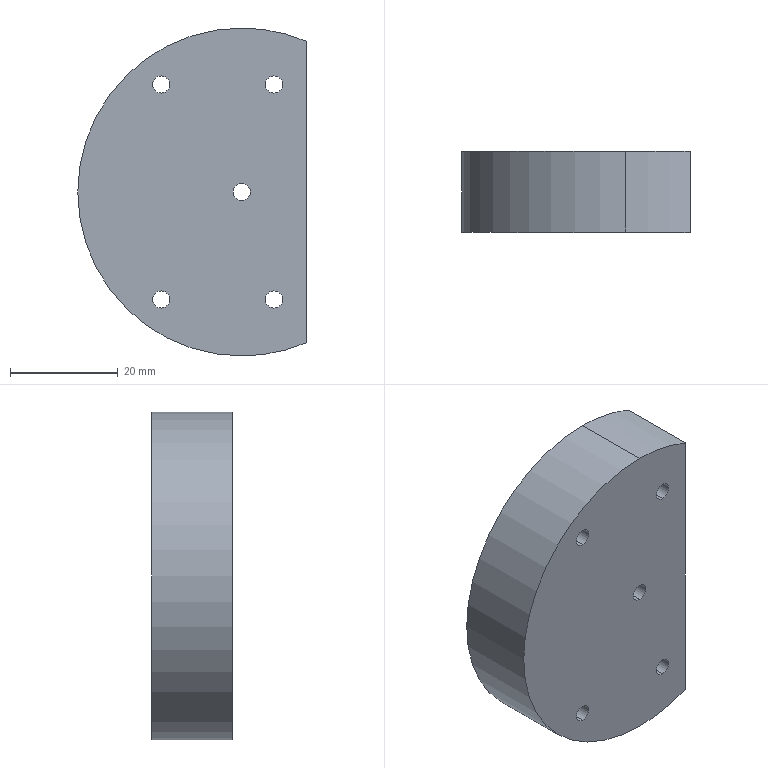Part | SolidWorks | features BaseBody 1 | 1 solid | 23 faces | box 42.5 x 15 x 61 mm | volume 7856 mm3 | cylinder 16 | plane 4 | spline 3 | commonest cylinder face diameters 3.2 x10 59 x3 61 x3
STEP:
#1=CARTESIAN_POINT('',(-15.,0.,21.6));
#2=VERTEX_POINT('',#1);
#3=CARTESIAN_POINT('',(-15.,0.,18.4));
#4=VERTEX_POINT('',#3);
#5=CARTESIAN_POINT('',(-15.,0.,20.));
#6=DIRECTION('',(0.,-1.,0.));
#7=DIRECTION('',(0.,0.,1.));
#8=AXIS2_PLACEMENT_3D('',#5,#6,#7);
#9=CIRCLE('',#8,1.6);
#10=EDGE_CURVE('',#2,#4,#9,.T.);
#11=ORIENTED_EDGE('',*,*,#10,.T.);
#12=CARTESIAN_POINT('',(-15.,3.,18.4));
#13=VERTEX_POINT('',#12);
#14=CARTESIAN_POINT('',(-15.,0.,18.4));
#15=DIRECTION('',(0.,1.,0.));
#16=VECTOR('',#15,1000.);
#17=LINE('',#14,#16);
#18=EDGE_CURVE('',#4,#13,#17,.T.);
#19=ORIENTED_EDGE('',*,*,#18,.T.);
#20=CARTESIAN_POINT('',(-15.,3.,21.6));
#21=VERTEX_POINT('',#20);
#22=CARTESIAN_POINT('',(-15.,3.,20.));
#23=DIRECTION('',(0.,1.,0.));
#24=DIRECTION('',(0.,0.,1.));
#25=AXIS2_PLACEMENT_3D('',#22,#23,#24);
#26=CIRCLE('',#25,1.6);
#27=EDGE_CURVE('',#13,#21,#26,.T.);
#28=ORIENTED_EDGE('',*,*,#27,.T.);
#29=CARTESIAN_POINT('',(-15.,0.,21.6));
#30=DIRECTION('',(0.,1.,0.));
#31=VECTOR('',#30,1000.);
#32=LINE('',#29,#31);
#33=EDGE_CURVE('',#2,#21,#32,.T.);
#34=ORIENTED_EDGE('',*,*,#33,.F.);
#35=EDGE_LOOP('',(#11,#19,#28,#34));
#36=FACE_OUTER_BOUND('',#35,.T.);
#37=CARTESIAN_POINT('',(-15.,0.,20.));
#38=DIRECTION('',(0.,1.,0.));
#39=DIRECTION('',(0.,0.,1.));
#40=AXIS2_PLACEMENT_3D('',#37,#38,#39);
#41=CYLINDRICAL_SURFACE('',#40,1.6);
#42=ADVANCED_FACE('',(#36),#41,.F.);
#43=CARTESIAN_POINT('',(6.,0.,18.4));
#44=VERTEX_POINT('',#43);
#45=CARTESIAN_POINT('',(6.,0.,21.6));
#46=VERTEX_POINT('',#45);
#47=CARTESIAN_POINT('',(6.,0.,20.));
#48=DIRECTION('',(0.,1.,0.));
#49=DIRECTION('',(0.,0.,1.));
#50=AXIS2_PLACEMENT_3D('',#47,#48,#49);
#51=CIRCLE('',#50,1.6);
#52=EDGE_CURVE('',#44,#46,#51,.T.);
#53=ORIENTED_EDGE('',*,*,#52,.F.);
#54=CARTESIAN_POINT('',(6.,3.,18.4));
#55=VERTEX_POINT('',#54);
#56=CARTESIAN_POINT('',(6.,0.,18.4));
#57=DIRECTION('',(0.,1.,0.));
#58=VECTOR('',#57,1000.);
#59=LINE('',#56,#58);
#60=EDGE_CURVE('',#44,#55,#59,.T.);
#61=ORIENTED_EDGE('',*,*,#60,.T.);
#62=CARTESIAN_POINT('',(6.,3.,21.6));
#63=VERTEX_POINT('',#62);
#64=CARTESIAN_POINT('',(6.,3.,20.));
#65=DIRECTION('',(0.,-1.,0.));
#66=DIRECTION('',(0.,0.,1.));
#67=AXIS2_PLACEMENT_3D('',#64,#65,#66);
#68=CIRCLE('',#67,1.6);
#69=EDGE_CURVE('',#63,#55,#68,.T.);
#70=ORIENTED_EDGE('',*,*,#69,.F.);
#71=CARTESIAN_POINT('',(6.,0.,21.6));
#72=DIRECTION('',(0.,1.,0.));
#73=VECTOR('',#72,1000.);
#74=LINE('',#71,#73);
#75=EDGE_CURVE('',#46,#63,#74,.T.);
#76=ORIENTED_EDGE('',*,*,#75,.F.);
#77=EDGE_LOOP('',(#53,#61,#70,#76));
#78=FACE_OUTER_BOUND('',#77,.T.);
#79=CARTESIAN_POINT('',(6.,0.,20.));
#80=DIRECTION('',(0.,1.,0.));
#81=DIRECTION('',(0.,0.,1.));
#82=AXIS2_PLACEMENT_3D('',#79,#80,#81);
#83=CYLINDRICAL_SURFACE('',#82,1.6);
#84=ADVANCED_FACE('',(#78),#83,.F.);
#85=CARTESIAN_POINT('',(6.,0.,-21.6));
#86=VERTEX_POINT('',#85);
#87=CARTESIAN_POINT('',(6.,0.,-18.4));
#88=VERTEX_POINT('',#87);
#89=CARTESIAN_POINT('',(6.,0.,-20.));
#90=DIRECTION('',(0.,1.,0.));
#91=DIRECTION('',(0.,0.,1.));
#92=AXIS2_PLACEMENT_3D('',#89,#90,#91);
#93=CIRCLE('',#92,1.6);
#94=EDGE_CURVE('',#86,#88,#93,.T.);
#95=ORIENTED_EDGE('',*,*,#94,.F.);
#96=CARTESIAN_POINT('',(6.,3.,-21.6));
#97=VERTEX_POINT('',#96);
#98=CARTESIAN_POINT('',(6.,0.,-21.6));
#99=DIRECTION('',(0.,1.,0.));
#100=VECTOR('',#99,1000.);
#101=LINE('',#98,#100);
#102=EDGE_CURVE('',#86,#97,#101,.T.);
#103=ORIENTED_EDGE('',*,*,#102,.T.);
#104=CARTESIAN_POINT('',(6.,3.,-18.4));
#105=VERTEX_POINT('',#104);
#106=CARTESIAN_POINT('',(6.,3.,-20.));
#107=DIRECTION('',(0.,-1.,0.));
#108=DIRECTION('',(0.,0.,1.));
#109=AXIS2_PLACEMENT_3D('',#106,#107,#108);
#110=CIRCLE('',#109,1.6);
#111=EDGE_CURVE('',#105,#97,#110,.T.);
#112=ORIENTED_EDGE('',*,*,#111,.F.);
#113=CARTESIAN_POINT('',(6.,0.,-18.4));
#114=DIRECTION('',(0.,1.,0.));
#115=VECTOR('',#114,1000.);
#116=LINE('',#113,#115);
#117=EDGE_CURVE('',#88,#105,#116,.T.);
#118=ORIENTED_EDGE('',*,*,#117,.F.);
#119=EDGE_LOOP('',(#95,#103,#112,#118));
#120=FACE_OUTER_BOUND('',#119,.T.);
#121=CARTESIAN_POINT('',(6.,0.,-20.));
#122=DIRECTION('',(0.,1.,0.));
#123=DIRECTION('',(0.,0.,1.));
#124=AXIS2_PLACEMENT_3D('',#121,#122,#123);
#125=CYLINDRICAL_SURFACE('',#124,1.6);
#126=ADVANCED_FACE('',(#120),#125,.F.);
#127=CARTESIAN_POINT('',(0.,0.,-1.6));
#128=VERTEX_POINT('',#127);
#129=CARTESIAN_POINT('',(0.,0.,1.6));
#130=VERTEX_POINT('',#129);
#131=CARTESIAN_POINT('',(0.,0.,0.));
#132=DIRECTION('',(0.,1.,0.));
#133=DIRECTION('',(0.,0.,1.));
#134=AXIS2_PLACEMENT_3D('',#131,#132,#133);
#135=CIRCLE('',#134,1.6);
#136=EDGE_CURVE('',#128,#130,#135,.T.);
#137=ORIENTED_EDGE('',*,*,#136,.F.);
#138=CARTESIAN_POINT('',(0.,3.,-1.6));
#139=VERTEX_POINT('',#138);
#140=CARTESIAN_POINT('',(0.,0.,-1.6));
#141=DIRECTION('',(0.,1.,0.));
#142=VECTOR('',#141,1000.);
#143=LINE('',#140,#142);
#144=EDGE_CURVE('',#128,#139,#143,.T.);
#145=ORIENTED_EDGE('',*,*,#144,.T.);
#146=CARTESIAN_POINT('',(0.,3.,1.6));
#147=VERTEX_POINT('',#146);
#148=CARTESIAN_POINT('',(0.,3.,0.));
#149=DIRECTION('',(0.,-1.,0.));
#150=DIRECTION('',(0.,0.,1.));
#151=AXIS2_PLACEMENT_3D('',#148,#149,#150);
#152=CIRCLE('',#151,1.6);
#153=EDGE_CURVE('',#147,#139,#152,.T.);
#154=ORIENTED_EDGE('',*,*,#153,.F.);
#155=CARTESIAN_POINT('',(0.,0.,1.6));
#156=DIRECTION('',(0.,1.,0.));
#157=VECTOR('',#156,1000.);
#158=LINE('',#155,#157);
#159=EDGE_CURVE('',#130,#147,#158,.T.);
#160=ORIENTED_EDGE('',*,*,#159,.F.);
#161=EDGE_LOOP('',(#137,#145,#154,#160));
#162=FACE_OUTER_BOUND('',#161,.T.);
#163=CARTESIAN_POINT('',(0.,0.,0.));
#164=DIRECTION('',(0.,1.,0.));
#165=DIRECTION('',(0.,0.,1.));
#166=AXIS2_PLACEMENT_3D('',#163,#164,#165);
#167=CYLINDRICAL_SURFACE('',#166,1.6);
#168=ADVANCED_FACE('',(#162),#167,.F.);
#169=CARTESIAN_POINT('',(-15.,0.,-21.6));
#170=VERTEX_POINT('',#169);
#171=CARTESIAN_POINT('',(-15.,0.,-18.4));
#172=VERTEX_POINT('',#171);
#173=CARTESIAN_POINT('',(-15.,0.,-20.));
#174=DIRECTION('',(0.,1.,0.));
#175=DIRECTION('',(0.,0.,1.));
#176=AXIS2_PLACEMENT_3D('',#173,#174,#175);
#177=CIRCLE('',#176,1.6);
#178=EDGE_CURVE('',#170,#172,#177,.T.);
#179=ORIENTED_EDGE('',*,*,#178,.F.);
#180=CARTESIAN_POINT('',(-15.,3.,-21.6));
#181=VERTEX_POINT('',#180);
#182=CARTESIAN_POINT('',(-15.,0.,-21.6));
#183=DIRECTION('',(0.,1.,0.));
#184=VECTOR('',#183,1000.);
#185=LINE('',#182,#184);
#186=EDGE_CURVE('',#170,#181,#185,.T.);
#187=ORIENTED_EDGE('',*,*,#186,.T.);
#188=CARTESIAN_POINT('',(-15.,3.,-18.4));
#189=VERTEX_POINT('',#188);
#190=CARTESIAN_POINT('',(-15.,3.,-20.));
#191=DIRECTION('',(0.,-1.,0.));
#192=DIRECTION('',(0.,0.,1.));
#193=AXIS2_PLACEMENT_3D('',#190,#191,#192);
#194=CIRCLE('',#193,1.6);
#195=EDGE_CURVE('',#189,#181,#194,.T.);
#196=ORIENTED_EDGE('',*,*,#195,.F.);
#197=CARTESIAN_POINT('',(-15.,0.,-18.4));
#198=DIRECTION('',(0.,1.,0.));
#199=VECTOR('',#198,1000.);
#200=LINE('',#197,#199);
#201=EDGE_CURVE('',#172,#189,#200,.T.);
#202=ORIENTED_EDGE('',*,*,#201,.F.);
#203=EDGE_LOOP('',(#179,#187,#196,#202));
#204=FACE_OUTER_BOUND('',#203,.T.);
#205=CARTESIAN_POINT('',(-15.,0.,-20.));
#206=DIRECTION('',(0.,1.,0.));
#207=DIRECTION('',(0.,0.,1.));
#208=AXIS2_PLACEMENT_3D('',#205,#206,#207);
#209=CYLINDRICAL_SURFACE('',#208,1.6);
#210=ADVANCED_FACE('',(#204),#209,.F.);
#211=CARTESIAN_POINT('',(0.,0.,-30.5));
#212=VERTEX_POINT('',#211);
#213=CARTESIAN_POINT('',(12.,0.,-28.04));
#214=VERTEX_POINT('',#213);
#215=CARTESIAN_POINT('',(0.,0.,0.));
#216=DIRECTION('',(0.,-1.,0.));
#217=DIRECTION('',(0.,0.,1.));
#218=AXIS2_PLACEMENT_3D('',#215,#216,#217);
#219=CIRCLE('',#218,30.5);
#220=EDGE_CURVE('',#212,#214,#219,.T.);
#221=ORIENTED_EDGE('',*,*,#220,.F.);
#222=CARTESIAN_POINT('',(0.,15.,-30.5));
#223=VERTEX_POINT('',#222);
#224=CARTESIAN_POINT('',(0.,0.,-30.5));
#225=DIRECTION('',(0.,1.,0.));
#226=VECTOR('',#225,1000.);
#227=LINE('',#224,#226);
#228=EDGE_CURVE('',#212,#223,#227,.T.);
#229=ORIENTED_EDGE('',*,*,#228,.T.);
#230=CARTESIAN_POINT('',(12.,15.,-28.04));
#231=VERTEX_POINT('',#230);
#232=CARTESIAN_POINT('',(0.,15.,0.));
#233=DIRECTION('',(0.,1.,0.));
#234=DIRECTION('',(0.,0.,1.));
#235=AXIS2_PLACEMENT_3D('',#232,#233,#234);
#236=CIRCLE('',#235,30.5);
#237=EDGE_CURVE('',#231,#223,#236,.T.);
#238=ORIENTED_EDGE('',*,*,#237,.F.);
#239=CARTESIAN_POINT('',(12.,7.5,-28.04));
#240=DIRECTION('',(0.,-1.,0.));
#241=VECTOR('',#240,1000.);
#242=LINE('',#239,#241);
#243=EDGE_CURVE('',#231,#214,#242,.T.);
#244=ORIENTED_EDGE('',*,*,#243,.T.);
#245=EDGE_LOOP('',(#221,#229,#238,#244));
#246=FACE_OUTER_BOUND('',#245,.T.);
#247=CARTESIAN_POINT('',(0.,0.,0.));
#248=DIRECTION('',(0.,1.,0.));
#249=DIRECTION('',(0.,0.,1.));
#250=AXIS2_PLACEMENT_3D('',#247,#248,#249);
#251=CYLINDRICAL_SURFACE('',#250,30.5);
#252=ADVANCED_FACE('',(#246),#251,.T.);
#253=ORIENTED_EDGE('',*,*,#228,.F.);
#254=CARTESIAN_POINT('',(0.,0.,30.5));
#255=VERTEX_POINT('',#254);
#256=CARTESIAN_POINT('',(0.,0.,0.));
#257=DIRECTION('',(0.,-1.,0.));
#258=DIRECTION('',(0.,0.,1.));
#259=AXIS2_PLACEMENT_3D('',#256,#257,#258);
#260=CIRCLE('',#259,30.5);
#261=EDGE_CURVE('',#255,#212,#260,.T.);
#262=ORIENTED_EDGE('',*,*,#261,.F.);
#263=CARTESIAN_POINT('',(0.,15.,30.5));
#264=VERTEX_POINT('',#263);
#265=CARTESIAN_POINT('',(0.,0.,30.5));
#266=DIRECTION('',(0.,1.,0.));
#267=VECTOR('',#266,1000.);
#268=LINE('',#265,#267);
#269=EDGE_CURVE('',#255,#264,#268,.T.);
#270=ORIENTED_EDGE('',*,*,#269,.T.);
#271=CARTESIAN_POINT('',(0.,15.,0.));
#272=DIRECTION('',(0.,1.,0.));
#273=DIRECTION('',(0.,0.,1.));
#274=AXIS2_PLACEMENT_3D('',#271,#272,#273);
#275=CIRCLE('',#274,30.5);
#276=EDGE_CURVE('',#223,#264,#275,.T.);
#277=ORIENTED_EDGE('',*,*,#276,.F.);
#278=EDGE_LOOP('',(#253,#262,#270,#277));
#279=FACE_OUTER_BOUND('',#278,.T.);
#280=CARTESIAN_POINT('',(0.,0.,0.));
#281=DIRECTION('',(0.,1.,0.));
#282=DIRECTION('',(0.,0.,1.));
#283=AXIS2_PLACEMENT_3D('',#280,#281,#282);
#284=CYLINDRICAL_SURFACE('',#283,30.5);
#285=ADVANCED_FACE('',(#279),#284,.T.);
#286=CARTESIAN_POINT('',(0.,4.,29.5));
#287=VERTEX_POINT('',#286);
#288=CARTESIAN_POINT('',(-0.000000003,4.,-29.5));
#289=VERTEX_POINT('',#288);
#290=CARTESIAN_POINT('',(0.,4.,0.));
#291=DIRECTION('',(0.,-1.,0.));
#292=DIRECTION('',(1.,0.,0.));
#293=AXIS2_PLACEMENT_3D('',#290,#291,#292);
#294=CIRCLE('',#293,29.5);
#295=EDGE_CURVE('',#287,#289,#294,.T.);
#296=ORIENTED_EDGE('',*,*,#295,.T.);
#297=CARTESIAN_POINT('',(0.,15.,-29.5));
#298=VERTEX_POINT('',#297);
#299=CARTESIAN_POINT('',(0.,4.,-29.5));
#300=DIRECTION('',(0.,1.,0.));
#301=VECTOR('',#300,1000.);
#302=LINE('',#299,#301);
#303=EDGE_CURVE('',#289,#298,#302,.T.);
#304=ORIENTED_EDGE('',*,*,#303,.T.);
#305=CARTESIAN_POINT('',(0.,15.,29.5));
#306=VERTEX_POINT('',#305);
#307=CARTESIAN_POINT('',(0.,15.,0.));
#308=DIRECTION('',(0.,1.,0.));
#309=DIRECTION('',(0.,0.,1.));
#310=AXIS2_PLACEMENT_3D('',#307,#308,#309);
#311=CIRCLE('',#310,29.5);
#312=EDGE_CURVE('',#298,#306,#311,.T.);
#313=ORIENTED_EDGE('',*,*,#312,.T.);
#314=CARTESIAN_POINT('',(0.,4.,29.5));
#315=DIRECTION('',(0.,1.,0.));
#316=VECTOR('',#315,1000.);
#317=LINE('',#314,#316);
#318=EDGE_CURVE('',#287,#306,#317,.T.);
#319=ORIENTED_EDGE('',*,*,#318,.F.);
#320=EDGE_LOOP('',(#296,#304,#313,#319));
#321=FACE_OUTER_BOUND('',#320,.T.);
#322=CARTESIAN_POINT('',(0.,4.,0.));
#323=DIRECTION('',(0.,1.,0.));
#324=DIRECTION('',(0.,0.,1.));
#325=AXIS2_PLACEMENT_3D('',#322,#323,#324);
#326=CYLINDRICAL_SURFACE('',#325,29.5);
#327=ADVANCED_FACE('',(#321),#326,.F.);
#328=CARTESIAN_POINT('',(12.,4.,26.949));
#329=VERTEX_POINT('',#328);
#330=CARTESIAN_POINT('',(0.,4.,0.000000001));
#331=DIRECTION('',(0.,-1.,0.));
#332=DIRECTION('',(0.,0.,-1.));
#333=AXIS2_PLACEMENT_3D('',#330,#331,#332);
#334=CIRCLE('',#333,29.5);
#335=EDGE_CURVE('',#329,#287,#334,.T.);
#336=ORIENTED_EDGE('',*,*,#335,.T.);
#337=ORIENTED_EDGE('',*,*,#318,.T.);
#338=CARTESIAN_POINT('',(12.,15.,26.949));
#339=VERTEX_POINT('',#338);
#340=CARTESIAN_POINT('',(0.,15.,0.));
#341=DIRECTION('',(0.,1.,0.));
#342=DIRECTION('',(0.,0.,1.));
#343=AXIS2_PLACEMENT_3D('',#340,#341,#342);
#344=CIRCLE('',#343,29.5);
#345=EDGE_CURVE('',#306,#339,#344,.T.);
#346=ORIENTED_EDGE('',*,*,#345,.T.);
#347=CARTESIAN_POINT('',(12.,7.5,26.949));
#348=DIRECTION('',(0.,-1.,0.));
#349=VECTOR('',#348,1000.);
#350=LINE('',#347,#349);
#351=EDGE_CURVE('',#339,#329,#350,.T.);
#352=ORIENTED_EDGE('',*,*,#351,.T.);
#353=EDGE_LOOP('',(#336,#337,#346,#352));
#354=FACE_OUTER_BOUND('',#353,.T.);
#355=CARTESIAN_POINT('',(0.,4.,0.));
#356=DIRECTION('',(0.,1.,0.));
#357=DIRECTION('',(0.,0.,1.));
#358=AXIS2_PLACEMENT_3D('',#355,#356,#357);
#359=CYLINDRICAL_SURFACE('',#358,29.5);
#360=ADVANCED_FACE('',(#354),#359,.F.);
#361=ORIENTED_EDGE('',*,*,#18,.F.);
#362=CARTESIAN_POINT('',(-15.,0.,20.));
#363=DIRECTION('',(0.,-1.,0.));
#364=DIRECTION('',(0.,0.,1.));
#365=AXIS2_PLACEMENT_3D('',#362,#363,#364);
#366=CIRCLE('',#365,1.6);
#367=EDGE_CURVE('',#4,#2,#366,.T.);
#368=ORIENTED_EDGE('',*,*,#367,.T.);
#369=ORIENTED_EDGE('',*,*,#33,.T.);
#370=CARTESIAN_POINT('',(-15.,3.,20.));
#371=DIRECTION('',(0.,1.,0.));
#372=DIRECTION('',(0.,0.,1.));
#373=AXIS2_PLACEMENT_3D('',#370,#371,#372);
#374=CIRCLE('',#373,1.6);
#375=EDGE_CURVE('',#21,#13,#374,.T.);
#376=ORIENTED_EDGE('',*,*,#375,.T.);
#377=EDGE_LOOP('',(#361,#368,#369,#376));
#378=FACE_OUTER_BOUND('',#377,.T.);
#379=CARTESIAN_POINT('',(-15.,0.,20.));
#380=DIRECTION('',(0.,1.,0.));
#381=DIRECTION('',(0.,0.,1.));
#382=AXIS2_PLACEMENT_3D('',#379,#380,#381);
#383=CYLINDRICAL_SURFACE('',#382,1.6);
#384=ADVANCED_FACE('',(#378),#383,.F.);
#385=ORIENTED_EDGE('',*,*,#69,.T.);
#386=CARTESIAN_POINT('',(6.,3.,20.));
#387=DIRECTION('',(0.,-1.,0.));
#388=DIRECTION('',(0.,0.,1.));
#389=AXIS2_PLACEMENT_3D('',#386,#387,#388);
#390=CIRCLE('',#389,1.6);
#391=EDGE_CURVE('',#55,#63,#390,.T.);
#392=ORIENTED_EDGE('',*,*,#391,.T.);
#393=EDGE_LOOP('',(#385,#392));
#394=FACE_BOUND('',#393,.T.);
#395=ORIENTED_EDGE('',*,*,#111,.T.);
#396=CARTESIAN_POINT('',(6.,3.,-20.));
#397=DIRECTION('',(0.,-1.,0.));
#398=DIRECTION('',(0.,0.,1.));
#399=AXIS2_PLACEMENT_3D('',#396,#397,#398);
#400=CIRCLE('',#399,1.6);
#401=EDGE_CURVE('',#97,#105,#400,.T.);
#402=ORIENTED_EDGE('',*,*,#401,.T.);
#403=EDGE_LOOP('',(#395,#402));
#404=FACE_BOUND('',#403,.T.);
#405=ORIENTED_EDGE('',*,*,#153,.T.);
#406=CARTESIAN_POINT('',(0.,3.,0.));
#407=DIRECTION('',(0.,-1.,0.));
#408=DIRECTION('',(0.,0.,1.));
#409=AXIS2_PLACEMENT_3D('',#406,#407,#408);
#410=CIRCLE('',#409,1.6);
#411=EDGE_CURVE('',#139,#147,#410,.T.);
#412=ORIENTED_EDGE('',*,*,#411,.T.);
#413=EDGE_LOOP('',(#405,#412));
#414=FACE_BOUND('',#413,.T.);
#415=ORIENTED_EDGE('',*,*,#195,.T.);
#416=CARTESIAN_POINT('',(-15.,3.,-20.));
#417=DIRECTION('',(0.,-1.,0.));
#418=DIRECTION('',(0.,0.,1.));
#419=AXIS2_PLACEMENT_3D('',#416,#417,#418);
#420=CIRCLE('',#419,1.6);
#421=EDGE_CURVE('',#181,#189,#420,.T.);
#422=ORIENTED_EDGE('',*,*,#421,.T.);
#423=EDGE_LOOP('',(#415,#422));
#424=FACE_BOUND('',#423,.T.);
#425=ORIENTED_EDGE('',*,*,#375,.F.);
#426=ORIENTED_EDGE('',*,*,#27,.F.);
#427=EDGE_LOOP('',(#425,#426));
#428=FACE_BOUND('',#427,.T.);
#429=CARTESIAN_POINT('',(-0.000000007,3.,-28.5));
#430=VERTEX_POINT('',#429);
#431=CARTESIAN_POINT('',(-0.000000007,3.,28.5));
#432=VERTEX_POINT('',#431);
#433=CARTESIAN_POINT('',(-0.000000007,3.,-28.5));
#434=CARTESIAN_POINT('',(-0.6334,3.,-28.5));
#435=CARTESIAN_POINT('',(-1.581,3.,-28.468));
#436=CARTESIAN_POINT('',(-2.684,3.,-28.376));
#437=CARTESIAN_POINT('',(-3.234,3.,-28.317));
#438=CARTESIAN_POINT('',(-3.509,3.,-28.283));
#439=CARTESIAN_POINT('',(-3.646,3.,-28.266));
#440=CARTESIAN_POINT('',(-3.715,3.,-28.257));
#441=CARTESIAN_POINT('',(-3.744,3.,-28.253));
#442=CARTESIAN_POINT('',(-3.764,3.,-28.25));
#443=CARTESIAN_POINT('',(-3.772,3.,-28.249));
#444=CARTESIAN_POINT('',(-4.494,3.,-28.153));
#445=CARTESIAN_POINT('',(-5.551,3.,-27.97));
#446=CARTESIAN_POINT('',(-6.77,3.,-27.688));
#447=CARTESIAN_POINT('',(-7.376,3.,-27.53));
#448=CARTESIAN_POINT('',(-7.678,3.,-27.446));
#449=CARTESIAN_POINT('',(-7.829,3.,-27.404));
#450=CARTESIAN_POINT('',(-7.905,3.,-27.382));
#451=CARTESIAN_POINT('',(-7.937,3.,-27.373));
#452=CARTESIAN_POINT('',(-7.958,3.,-27.366));
#453=CARTESIAN_POINT('',(-7.968,3.,-27.364));
#454=CARTESIAN_POINT('',(-8.756,3.,-27.134));
#455=CARTESIAN_POINT('',(-9.902,3.,-26.746));
#456=CARTESIAN_POINT('',(-11.206,3.,-26.21));
#457=CARTESIAN_POINT('',(-11.85,3.,-25.921));
#458=CARTESIAN_POINT('',(-12.17,3.,-25.771));
#459=CARTESIAN_POINT('',(-12.33,3.,-25.695));
#460=CARTESIAN_POINT('',(-12.398,3.,-25.662));
#461=CARTESIAN_POINT('',(-12.443,3.,-25.64));
#462=CARTESIAN_POINT('',(-12.464,3.,-25.63));
#463=CARTESIAN_POINT('',(-12.883,3.,-25.426));
#464=CARTESIAN_POINT('',(-13.468,3.,-25.124));
#465=CARTESIAN_POINT('',(-14.138,3.,-24.748));
#466=CARTESIAN_POINT('',(-14.47,3.,-24.554));
#467=CARTESIAN_POINT('',(-14.635,3.,-24.455));
#468=CARTESIAN_POINT('',(-14.706,3.,-24.413));
#469=CARTESIAN_POINT('',(-14.753,3.,-24.385));
#470=CARTESIAN_POINT('',(-14.775,3.,-24.371));
#471=CARTESIAN_POINT('',(-15.196,3.,-24.116));
#472=CARTESIAN_POINT('',(-15.78,3.,-23.741));
#473=CARTESIAN_POINT('',(-16.445,3.,-23.279));
#474=CARTESIAN_POINT('',(-16.774,3.,-23.041));
#475=CARTESIAN_POINT('',(-16.937,3.,-22.921));
#476=CARTESIAN_POINT('',(-17.007,3.,-22.869));
#477=CARTESIAN_POINT('',(-17.054,3.,-22.835));
#478=CARTESIAN_POINT('',(-17.076,3.,-22.818));
#479=CARTESIAN_POINT('',(-17.49,3.,-22.508));
#480=CARTESIAN_POINT('',(-18.062,3.,-22.055));
#481=CARTESIAN_POINT('',(-18.709,3.,-21.502));
#482=CARTESIAN_POINT('',(-19.028,3.,-21.218));
#483=CARTESIAN_POINT('',(-19.186,3.,-21.075));
#484=CARTESIAN_POINT('',(-19.253,3.,-21.014));
#485=CARTESIAN_POINT('',(-19.298,3.,-20.972));
#486=CARTESIAN_POINT('',(-19.319,3.,-20.953));
#487=CARTESIAN_POINT('',(-19.717,3.,-20.585));
#488=CARTESIAN_POINT('',(-20.264,3.,-20.052));
#489=CARTESIAN_POINT('',(-20.877,3.,-19.404));
#490=CARTESIAN_POINT('',(-21.177,3.,-19.074));
#491=CARTESIAN_POINT('',(-21.325,3.,-18.907));
#492=CARTESIAN_POINT('',(-21.389,3.,-18.836));
#493=CARTESIAN_POINT('',(-21.431,3.,-18.788));
#494=CARTESIAN_POINT('',(-21.451,3.,-18.765));
#495=CARTESIAN_POINT('',(-21.822,3.,-18.339));
#496=CARTESIAN_POINT('',(-22.328,3.,-17.725));
#497=CARTESIAN_POINT('',(-22.889,3.,-16.985));
#498=CARTESIAN_POINT('',(-23.161,3.,-16.608));
#499=CARTESIAN_POINT('',(-23.296,3.,-16.418));
#500=CARTESIAN_POINT('',(-23.353,3.,-16.337));
#501=CARTESIAN_POINT('',(-23.391,3.,-16.282));
#502=CARTESIAN_POINT('',(-23.409,3.,-16.256));
#503=CARTESIAN_POINT('',(-23.742,3.,-15.775));
#504=CARTESIAN_POINT('',(-24.192,3.,-15.084));
#505=CARTESIAN_POINT('',(-24.682,3.,-14.255));
#506=CARTESIAN_POINT('',(-24.917,3.,-13.835));
#507=CARTESIAN_POINT('',(-25.016,3.,-13.654));
#508=CARTESIAN_POINT('',(-25.082,3.,-13.533));
#509=CARTESIAN_POINT('',(-25.114,3.,-13.474));
#510=CARTESIAN_POINT('',(-25.414,3.,-12.911));
#511=CARTESIAN_POINT('',(-25.791,3.,-12.15));
#512=CARTESIAN_POINT('',(-26.191,3.,-11.244));
#513=CARTESIAN_POINT('',(-26.381,3.,-10.786));
#514=CARTESIAN_POINT('',(-26.46,3.,-10.588));
#515=CARTESIAN_POINT('',(-26.513,3.,-10.457));
#516=CARTESIAN_POINT('',(-26.538,3.,-10.392));
#517=CARTESIAN_POINT('',(-26.774,3.,-9.784));
#518=CARTESIAN_POINT('',(-27.064,3.,-8.965));
#519=CARTESIAN_POINT('',(-27.358,3.,-7.995));
#520=CARTESIAN_POINT('',(-27.475,3.,-7.576));
#521=CARTESIAN_POINT('',(-27.551,3.,-7.296));
#522=CARTESIAN_POINT('',(-27.587,3.,-7.158));
#523=CARTESIAN_POINT('',(-27.768,3.,-6.445));
#524=CARTESIAN_POINT('',(-27.959,3.,-5.583));
#525=CARTESIAN_POINT('',(-28.109,3.,-4.714));
#526=CARTESIAN_POINT('',(-28.2,3.,-4.133));
#527=CARTESIAN_POINT('',(-28.241,3.,-3.843));
#528=CARTESIAN_POINT('',(-28.426,3.,-2.371));
#529=CARTESIAN_POINT('',(-28.5,3.,-1.187));
#530=CARTESIAN_POINT('',(-28.5,3.,0.5936));
#531=CARTESIAN_POINT('',(-28.472,3.,1.482));
#532=CARTESIAN_POINT('',(-28.391,3.,2.516));
#533=CARTESIAN_POINT('',(-28.346,3.,2.959));
#534=CARTESIAN_POINT('',(-28.314,3.,3.254));
#535=CARTESIAN_POINT('',(-28.297,3.,3.403));
#536=CARTESIAN_POINT('',(-28.205,3.,4.133));
#537=CARTESIAN_POINT('',(-28.068,3.,5.005));
#538=CARTESIAN_POINT('',(-27.861,3.,6.013));
#539=CARTESIAN_POINT('',(-27.746,3.,6.515));
#540=CARTESIAN_POINT('',(-27.694,3.,6.73));
#541=CARTESIAN_POINT('',(-27.659,3.,6.873));
#542=CARTESIAN_POINT('',(-27.641,3.,6.945));
#543=CARTESIAN_POINT('',(-27.48,3.,7.578));
#544=CARTESIAN_POINT('',(-27.241,3.,8.413));
#545=CARTESIAN_POINT('',(-26.917,3.,9.373));
#546=CARTESIAN_POINT('',(-26.744,3.,9.85));
#547=CARTESIAN_POINT('',(-26.668,3.,10.054));
#548=CARTESIAN_POINT('',(-26.616,3.,10.189));
#549=CARTESIAN_POINT('',(-26.59,3.,10.258));
#550=CARTESIAN_POINT('',(-26.359,3.,10.853));
#551=CARTESIAN_POINT('',(-26.028,3.,11.635));
#552=CARTESIAN_POINT('',(-25.601,3.,12.53));
#553=CARTESIAN_POINT('',(-25.377,3.,12.972));
#554=CARTESIAN_POINT('',(-25.279,3.,13.161));
#555=CARTESIAN_POINT('',(-25.214,3.,13.287));
#556=CARTESIAN_POINT('',(-25.179,3.,13.351));
#557=CARTESIAN_POINT('',(-24.888,3.,13.898));
#558=CARTESIAN_POINT('',(-24.479,3.,14.614));
#559=CARTESIAN_POINT('',(-23.966,3.,15.428));
#560=CARTESIAN_POINT('',(-23.7,3.,15.83));
#561=CARTESIAN_POINT('',(-23.565,3.,16.029));
#562=CARTESIAN_POINT('',(-23.507,3.,16.114));
#563=CARTESIAN_POINT('',(-23.468,3.,16.171));
#564=CARTESIAN_POINT('',(-23.448,3.,16.2));
#565=CARTESIAN_POINT('',(-23.126,3.,16.665));
#566=CARTESIAN_POINT('',(-22.655,3.,17.306));
#567=CARTESIAN_POINT('',(-22.074,3.,18.031));
#568=CARTESIAN_POINT('',(-21.776,3.,18.387));
#569=CARTESIAN_POINT('',(-21.625,3.,18.564));
#570=CARTESIAN_POINT('',(-21.56,3.,18.639));
#571=CARTESIAN_POINT('',(-21.516,3.,18.69));
#572=CARTESIAN_POINT('',(-21.494,3.,18.716));
#573=CARTESIAN_POINT('',(-21.137,3.,19.124));
#574=CARTESIAN_POINT('',(-20.62,3.,19.686));
#575=CARTESIAN_POINT('',(-19.99,3.,20.317));
#576=CARTESIAN_POINT('',(-19.668,3.,20.626));
#577=CARTESIAN_POINT('',(-19.506,3.,20.779));
#578=CARTESIAN_POINT('',(-19.436,3.,20.844));
#579=CARTESIAN_POINT('',(-19.389,3.,20.888));
#580=CARTESIAN_POINT('',(-19.365,3.,20.91));
#581=CARTESIAN_POINT('',(-18.985,3.,21.262));
#582=CARTESIAN_POINT('',(-18.436,3.,21.743));
#583=CARTESIAN_POINT('',(-17.775,3.,22.28));
#584=CARTESIAN_POINT('',(-17.439,3.,22.542));
#585=CARTESIAN_POINT('',(-17.27,3.,22.672));
#586=CARTESIAN_POINT('',(-17.197,3.,22.727));
#587=CARTESIAN_POINT('',(-17.149,3.,22.763));
#588=CARTESIAN_POINT('',(-17.123,3.,22.783));
#589=CARTESIAN_POINT('',(-16.729,3.,23.078));
#590=CARTESIAN_POINT('',(-16.164,3.,23.481));
#591=CARTESIAN_POINT('',(-15.487,3.,23.927));
#592=CARTESIAN_POINT('',(-15.145,3.,24.143));
#593=CARTESIAN_POINT('',(-14.973,3.,24.25));
#594=CARTESIAN_POINT('',(-14.899,3.,24.296));
#595=CARTESIAN_POINT('',(-14.849,3.,24.326));
#596=CARTESIAN_POINT('',(-14.823,3.,24.342));
#597=CARTESIAN_POINT('',(-14.424,3.,24.584));
#598=CARTESIAN_POINT('',(-13.854,3.,24.913));
#599=CARTESIAN_POINT('',(-13.176,3.,25.273));
#600=CARTESIAN_POINT('',(-12.833,3.,25.448));
#601=CARTESIAN_POINT('',(-12.661,3.,25.533));
#602=CARTESIAN_POINT('',(-12.587,3.,25.57));
#603=CARTESIAN_POINT('',(-12.538,3.,25.594));
#604=CARTESIAN_POINT('',(-12.511,3.,25.607));
#605=CARTESIAN_POINT('',(-11.762,3.,25.972));
#606=CARTESIAN_POINT('',(-10.654,3.,26.456));
#607=CARTESIAN_POINT('',(-9.328,3.,26.936));
#608=CARTESIAN_POINT('',(-8.657,3.,27.155));
#609=CARTESIAN_POINT('',(-8.319,3.,27.259));
#610=CARTESIAN_POINT('',(-8.15,3.,27.31));
#611=CARTESIAN_POINT('',(-8.065,3.,27.335));
#612=CARTESIAN_POINT('',(-8.029,3.,27.346));
#613=CARTESIAN_POINT('',(-8.004,3.,27.353));
#614=CARTESIAN_POINT('',(-7.991,3.,27.357));
#615=CARTESIAN_POINT('',(-7.292,3.,27.561));
#616=CARTESIAN_POINT('',(-6.251,3.,27.822));
#617=CARTESIAN_POINT('',(-5.022,3.,28.058));
#618=CARTESIAN_POINT('',(-4.404,3.,28.159));
#619=CARTESIAN_POINT('',(-4.094,3.,28.205));
#620=CARTESIAN_POINT('',(-3.939,3.,28.227));
#621=CARTESIAN_POINT('',(-3.861,3.,28.237));
#622=CARTESIAN_POINT('',(-3.828,3.,28.242));
#623=CARTESIAN_POINT('',(-3.805,3.,28.245));
#624=CARTESIAN_POINT('',(-3.793,3.,28.246));
#625=CARTESIAN_POINT('',(-2.528,3.,28.416));
#626=CARTESIAN_POINT('',(-1.267,3.,28.5));
#627=CARTESIAN_POINT('',(-0.000000007,3.,28.5));
#628=B_SPLINE_CURVE_WITH_KNOTS('',3,(#433,#434,#435,#436,#437,#438,#439,#440,#441,#442,#443,#444,#445,#446,#447,#448,#449,#450,#451,#452,#453,#454,#455,#456,#457,#458,#459,#460,#461,#462,#463,#464,#465,#466,#467,#468,#469,#470,#471,#472,#473,#474,#475,#476,#477,#478,#479,#480,#481,#482,#483,#484,#485,#486,#487,#488,#489,#490,#491,#492,#493,#494,#495,#496,#497,#498,#499,#500,#501,#502,#503,#504,#505,#506,#507,#508,#509,#510,#511,#512,#513,#514,#515,#516,#517,#518,#519,#520,#521,#522,#523,#524,#525,#526,#527,#528,#529,#530,#531,#532,#533,#534,#535,#536,#537,#538,#539,#540,#541,#542,#543,#544,#545,#546,#547,#548,#549,#550,#551,#552,#553,#554,#555,#556,#557,#558,#559,#560,#561,#562,#563,#564,#565,#566,#567,#568,#569,#570,#571,#572,#573,#574,#575,#576,#577,#578,#579,#580,#581,#582,#583,#584,#585,#586,#587,#588,#589,#590,#591,#592,#593,#594,#595,#596,#597,#598,#599,#600,#601,#602,#603,#604,#605,#606,#607,#608,#609,#610,#611,#612,#613,#614,#615,#616,#617,#618,#619,#620,#621,#622,#623,#624,#625,#626,#627),.UNSPECIFIED.,.F.,.F.,(4,1,1,1,1,1,1,2,2,1,1,1,1,1,1,2,2,1,1,1,1,1,2,2,1,1,1,1,2,2,1,1,1,1,2,2,1,1,1,1,2,2,1,1,1,1,2,2,1,1,1,1,2,2,1,1,1,2,2,1,1,1,2,2,1,1,2,2,1,2,2,2,1,1,2,2,1,1,1,2,2,1,1,1,2,2,1,1,1,2,2,1,1,1,1,2,2,1,1,1,1,2,2,1,1,1,1,2,2,1,1,1,1,2,2,1,1,1,1,2,2,1,1,1,1,2,2,1,1,1,1,1,1,2,2,1,1,1,1,1,1,2,2,4),(0.,0.03125,0.04687,0.05469,0.05859,0.06055,0.06152,0.06201,0.0625,0.09375,0.1094,0.1172,0.1211,0.123,0.124,0.1245,0.125,0.1562,0.1719,0.1797,0.1836,0.1855,0.1865,0.1875,0.2031,0.2109,0.2148,0.2168,0.2178,0.2187,0.2344,0.2422,0.2461,0.248,0.249,0.25,0.2656,0.2734,0.2773,0.2793,0.2803,0.2812,0.2969,0.3047,0.3086,0.3105,0.3115,0.3125,0.3281,0.3359,0.3398,0.3418,0.3428,0.3437,0.3594,0.3672,0.3711,0.373,0.375,0.3906,0.3984,0.4023,0.4043,0.4062,0.4219,0.4297,0.4336,0.4375,0.4531,0.4609,0.4687,0.5,0.5156,0.5234,0.5273,0.5312,0.5469,0.5547,0.5586,0.5605,0.5625,0.5781,0.5859,0.5898,0.5918,0.5937,0.6094,0.6172,0.6211,0.623,0.625,0.6406,0.6484,0.6523,0.6543,0.6553,0.6562,0.6719,0.6797,0.6836,0.6855,0.6865,0.6875,0.7031,0.7109,0.7148,0.7168,0.7178,0.7187,0.7344,0.7422,0.7461,0.748,0.749,0.75,0.7656,0.7734,0.7773,0.7793,0.7803,0.7812,0.7969,0.8047,0.8086,0.8105,0.8115,0.8125,0.8437,0.8594,0.8672,0.8711,0.873,0.874,0.8745,0.875,0.9062,0.9219,0.9297,0.9336,0.9355,0.9365,0.937,0.9375,1.),.UNSPECIFIED.);
#629=EDGE_CURVE('',#430,#432,#628,.T.);
#630=ORIENTED_EDGE('',*,*,#629,.T.);
#631=CARTESIAN_POINT('',(12.,3.,25.851));
#632=VERTEX_POINT('',#631);
#633=CARTESIAN_POINT('',(-0.000000007,3.,28.5));
#634=CARTESIAN_POINT('',(0.5151,3.,28.5));
#635=CARTESIAN_POINT('',(1.287,3.,28.479));
#636=CARTESIAN_POINT('',(2.056,3.,28.427));
#637=CARTESIAN_POINT('',(2.569,3.,28.385));
#638=CARTESIAN_POINT('',(2.824,3.,28.361));
#639=CARTESIAN_POINT('',(4.111,3.,28.221));
#640=CARTESIAN_POINT('',(5.132,3.,28.053));
#641=CARTESIAN_POINT('',(6.65,3.,27.718));
#642=CARTESIAN_POINT('',(7.403,3.,27.53));
#643=CARTESIAN_POINT('',(8.148,3.,27.312));
#644=CARTESIAN_POINT('',(8.643,3.,27.159));
#645=CARTESIAN_POINT('',(8.891,3.,27.079));
#646=CARTESIAN_POINT('',(10.11,3.,26.667));
#647=CARTESIAN_POINT('',(11.065,3.,26.285));
#648=CARTESIAN_POINT('',(12.,3.,25.851));
#649=B_SPLINE_CURVE_WITH_KNOTS('',3,(#633,#634,#635,#636,#637,#638,#639,#640,#641,#642,#643,#644,#645,#646,#647,#648),.UNSPECIFIED.,.F.,.F.,(4,1,2,2,2,1,2,2,4),(0.,0.125,0.1875,0.25,0.5,0.625,0.6875,0.75,1.),.UNSPECIFIED.);
#650=EDGE_CURVE('',#432,#632,#649,.T.);
#651=ORIENTED_EDGE('',*,*,#650,.T.);
#652=CARTESIAN_POINT('',(12.,3.,-25.851));
#653=VERTEX_POINT('',#652);
#654=CARTESIAN_POINT('',(12.,3.,0.));
#655=DIRECTION('',(0.,0.,-1.));
#656=VECTOR('',#655,1000.);
#657=LINE('',#654,#656);
#658=EDGE_CURVE('',#632,#653,#657,.T.);
#659=ORIENTED_EDGE('',*,*,#658,.T.);
#660=CARTESIAN_POINT('',(12.,3.,-25.851));
#661=CARTESIAN_POINT('',(11.533,3.,-26.067));
#662=CARTESIAN_POINT('',(10.824,3.,-26.373));
#663=CARTESIAN_POINT('',(10.104,3.,-26.65));
#664=CARTESIAN_POINT('',(9.621,3.,-26.828));
#665=CARTESIAN_POINT('',(9.38,3.,-26.914));
#666=CARTESIAN_POINT('',(8.153,3.,-27.329));
#667=CARTESIAN_POINT('',(7.156,3.,-27.607));
#668=CARTESIAN_POINT('',(5.638,3.,-27.942));
#669=CARTESIAN_POINT('',(4.876,3.,-28.088));
#670=CARTESIAN_POINT('',(4.109,3.,-28.204));
#671=CARTESIAN_POINT('',(3.596,3.,-28.273));
#672=CARTESIAN_POINT('',(3.337,3.,-28.305));
#673=CARTESIAN_POINT('',(2.058,3.,-28.444));
#674=CARTESIAN_POINT('',(1.031,3.,-28.5));
#675=CARTESIAN_POINT('',(-0.000000007,3.,-28.5));
#676=B_SPLINE_CURVE_WITH_KNOTS('',3,(#660,#661,#662,#663,#664,#665,#666,#667,#668,#669,#670,#671,#672,#673,#674,#675),.UNSPECIFIED.,.F.,.F.,(4,1,2,2,2,1,2,2,4),(0.,0.125,0.1875,0.25,0.5,0.625,0.6875,0.75,1.),.UNSPECIFIED.);
#677=EDGE_CURVE('',#653,#430,#676,.T.);
#678=ORIENTED_EDGE('',*,*,#677,.T.);
#679=EDGE_LOOP('',(#630,#651,#659,#678));
#680=FACE_OUTER_BOUND('',#679,.T.);
#681=CARTESIAN_POINT('',(-28.743,3.,-28.842));
#682=DIRECTION('',(0.,1.,0.));
#683=DIRECTION('',(0.,0.,1.));
#684=AXIS2_PLACEMENT_3D('',#681,#682,#683);
#685=PLANE('',#684);
#686=ADVANCED_FACE('',(#394,#404,#414,#424,#428,#680),#685,.T.);
#687=CARTESIAN_POINT('',(6.,0.,20.));
#688=DIRECTION('',(0.,1.,0.));
#689=DIRECTION('',(0.,0.,1.));
#690=AXIS2_PLACEMENT_3D('',#687,#688,#689);
#691=CIRCLE('',#690,1.6);
#692=EDGE_CURVE('',#46,#44,#691,.T.);
#693=ORIENTED_EDGE('',*,*,#692,.T.);
#694=ORIENTED_EDGE('',*,*,#52,.T.);
#695=EDGE_LOOP('',(#693,#694));
#696=FACE_BOUND('',#695,.T.);
#697=CARTESIAN_POINT('',(6.,0.,-20.));
#698=DIRECTION('',(0.,1.,0.));
#699=DIRECTION('',(0.,0.,1.));
#700=AXIS2_PLACEMENT_3D('',#697,#698,#699);
#701=CIRCLE('',#700,1.6);
#702=EDGE_CURVE('',#88,#86,#701,.T.);
#703=ORIENTED_EDGE('',*,*,#702,.T.);
#704=ORIENTED_EDGE('',*,*,#94,.T.);
#705=EDGE_LOOP('',(#703,#704));
#706=FACE_BOUND('',#705,.T.);
#707=CARTESIAN_POINT('',(0.,0.,0.));
#708=DIRECTION('',(0.,1.,0.));
#709=DIRECTION('',(0.,0.,1.));
#710=AXIS2_PLACEMENT_3D('',#707,#708,#709);
#711=CIRCLE('',#710,1.6);
#712=EDGE_CURVE('',#130,#128,#711,.T.);
#713=ORIENTED_EDGE('',*,*,#712,.T.);
#714=ORIENTED_EDGE('',*,*,#136,.T.);
#715=EDGE_LOOP('',(#713,#714));
#716=FACE_BOUND('',#715,.T.);
#717=CARTESIAN_POINT('',(-15.,0.,-20.));
#718=DIRECTION('',(0.,1.,0.));
#719=DIRECTION('',(0.,0.,1.));
#720=AXIS2_PLACEMENT_3D('',#717,#718,#719);
#721=CIRCLE('',#720,1.6);
#722=EDGE_CURVE('',#172,#170,#721,.T.);
#723=ORIENTED_EDGE('',*,*,#722,.T.);
#724=ORIENTED_EDGE('',*,*,#178,.T.);
#725=EDGE_LOOP('',(#723,#724));
#726=FACE_BOUND('',#725,.T.);
#727=ORIENTED_EDGE('',*,*,#10,.F.);
#728=ORIENTED_EDGE('',*,*,#367,.F.);
#729=EDGE_LOOP('',(#727,#728));
#730=FACE_BOUND('',#729,.T.);
#731=CARTESIAN_POINT('',(12.,0.,28.04));
#732=VERTEX_POINT('',#731);
#733=CARTESIAN_POINT('',(12.,0.,0.));
#734=DIRECTION('',(0.,0.,1.));
#735=VECTOR('',#734,1000.);
#736=LINE('',#733,#735);
#737=EDGE_CURVE('',#214,#732,#736,.T.);
#738=ORIENTED_EDGE('',*,*,#737,.T.);
#739=CARTESIAN_POINT('',(0.,0.,0.));
#740=DIRECTION('',(0.,-1.,0.));
#741=DIRECTION('',(0.,0.,1.));
#742=AXIS2_PLACEMENT_3D('',#739,#740,#741);
#743=CIRCLE('',#742,30.5);
#744=EDGE_CURVE('',#732,#255,#743,.T.);
#745=ORIENTED_EDGE('',*,*,#744,.T.);
#746=ORIENTED_EDGE('',*,*,#261,.T.);
#747=ORIENTED_EDGE('',*,*,#220,.T.);
#748=EDGE_LOOP('',(#738,#745,#746,#747));
#749=FACE_OUTER_BOUND('',#748,.T.);
#750=CARTESIAN_POINT('',(-30.755,0.,30.866));
#751=DIRECTION('',(0.,-1.,0.));
#752=DIRECTION('',(0.,0.,-1.));
#753=AXIS2_PLACEMENT_3D('',#750,#751,#752);
#754=PLANE('',#753);
#755=ADVANCED_FACE('',(#696,#706,#716,#726,#730,#749),#754,.T.);
#756=ORIENTED_EDGE('',*,*,#60,.F.);
#757=ORIENTED_EDGE('',*,*,#692,.F.);
#758=ORIENTED_EDGE('',*,*,#75,.T.);
#759=ORIENTED_EDGE('',*,*,#391,.F.);
#760=EDGE_LOOP('',(#756,#757,#758,#759));
#761=FACE_OUTER_BOUND('',#760,.T.);
#762=CARTESIAN_POINT('',(6.,0.,20.));
#763=DIRECTION('',(0.,1.,0.));
#764=DIRECTION('',(0.,0.,1.));
#765=AXIS2_PLACEMENT_3D('',#762,#763,#764);
#766=CYLINDRICAL_SURFACE('',#765,1.6);
#767=ADVANCED_FACE('',(#761),#766,.F.);
#768=ORIENTED_EDGE('',*,*,#102,.F.);
#769=ORIENTED_EDGE('',*,*,#702,.F.);
#770=ORIENTED_EDGE('',*,*,#117,.T.);
#771=ORIENTED_EDGE('',*,*,#401,.F.);
#772=EDGE_LOOP('',(#768,#769,#770,#771));
#773=FACE_OUTER_BOUND('',#772,.T.);
#774=CARTESIAN_POINT('',(6.,0.,-20.));
#775=DIRECTION('',(0.,1.,0.));
#776=DIRECTION('',(0.,0.,1.));
#777=AXIS2_PLACEMENT_3D('',#774,#775,#776);
#778=CYLINDRICAL_SURFACE('',#777,1.6);
#779=ADVANCED_FACE('',(#773),#778,.F.);
#780=ORIENTED_EDGE('',*,*,#144,.F.);
#781=ORIENTED_EDGE('',*,*,#712,.F.);
#782=ORIENTED_EDGE('',*,*,#159,.T.);
#783=ORIENTED_EDGE('',*,*,#411,.F.);
#784=EDGE_LOOP('',(#780,#781,#782,#783));
#785=FACE_OUTER_BOUND('',#784,.T.);
#786=CARTESIAN_POINT('',(0.,0.,0.));
#787=DIRECTION('',(0.,1.,0.));
#788=DIRECTION('',(0.,0.,1.));
#789=AXIS2_PLACEMENT_3D('',#786,#787,#788);
#790=CYLINDRICAL_SURFACE('',#789,1.6);
#791=ADVANCED_FACE('',(#785),#790,.F.);
#792=ORIENTED_EDGE('',*,*,#186,.F.);
#793=ORIENTED_EDGE('',*,*,#722,.F.);
#794=ORIENTED_EDGE('',*,*,#201,.T.);
#795=ORIENTED_EDGE('',*,*,#421,.F.);
#796=EDGE_LOOP('',(#792,#793,#794,#795));
#797=FACE_OUTER_BOUND('',#796,.T.);
#798=CARTESIAN_POINT('',(-15.,0.,-20.));
#799=DIRECTION('',(0.,1.,0.));
#800=DIRECTION('',(0.,0.,1.));
#801=AXIS2_PLACEMENT_3D('',#798,#799,#800);
#802=CYLINDRICAL_SURFACE('',#801,1.6);
#803=ADVANCED_FACE('',(#797),#802,.F.);
#804=CARTESIAN_POINT('',(0.,4.,29.5));
#805=CARTESIAN_POINT('',(0.,3.414,29.5));
#806=CARTESIAN_POINT('',(0.,3.,29.086));
#807=CARTESIAN_POINT('',(-0.000000007,3.,28.5));
#808=(BOUNDED_CURVE()B_SPLINE_CURVE(3,(#804,#805,#806,#807),.UNSPECIFIED.,.F.,.F.)B_SPLINE_CURVE_WITH_KNOTS((4,4),(0.06314,0.9369),.UNSPECIFIED.)CURVE()GEOMETRIC_REPRESENTATION_ITEM()RATIONAL_B_SPLINE_CURVE((0.9566,0.7698,0.7698,0.9566))REPRESENTATION_ITEM(''));
#809=EDGE_CURVE('',#287,#432,#808,.T.);
#810=ORIENTED_EDGE('',*,*,#809,.F.);
#811=ORIENTED_EDGE('',*,*,#335,.F.);
#812=CARTESIAN_POINT('',(12.,3.,25.851));
#813=CARTESIAN_POINT('',(12.,3.,25.989));
#814=CARTESIAN_POINT('',(12.,3.023,26.124));
#815=CARTESIAN_POINT('',(12.,3.117,26.385));
#816=CARTESIAN_POINT('',(12.,3.185,26.504));
#817=CARTESIAN_POINT('',(12.,3.366,26.713));
#818=CARTESIAN_POINT('',(12.,3.476,26.798));
#819=CARTESIAN_POINT('',(12.,3.725,26.917));
#820=CARTESIAN_POINT('',(12.,3.861,26.949));
#821=CARTESIAN_POINT('',(12.,4.,26.949));
#822=B_SPLINE_CURVE_WITH_KNOTS('',3,(#812,#813,#814,#815,#816,#817,#818,#819,#820,#821),.UNSPECIFIED.,.F.,.F.,(4,2,2,2,4),(0.,0.0004102,0.0008204,0.001231,0.001641),.UNSPECIFIED.);
#823=EDGE_CURVE('',#632,#329,#822,.T.);
#824=ORIENTED_EDGE('',*,*,#823,.F.);
#825=ORIENTED_EDGE('',*,*,#650,.F.);
#826=EDGE_LOOP('',(#810,#811,#824,#825));
#827=FACE_OUTER_BOUND('',#826,.T.);
#828=CARTESIAN_POINT('',(0.,4.1,29.495));
#829=CARTESIAN_POINT('',(4.333,4.1,29.495));
#830=CARTESIAN_POINT('',(8.563,4.1,28.555));
#831=CARTESIAN_POINT('',(12.489,4.1,26.721));
#832=CARTESIAN_POINT('',(0.,3.42,29.563));
#833=CARTESIAN_POINT('',(4.343,3.42,29.563));
#834=CARTESIAN_POINT('',(8.583,3.42,28.621));
#835=CARTESIAN_POINT('',(12.518,3.42,26.782));
#836=CARTESIAN_POINT('',(0.,2.937,29.08));
#837=CARTESIAN_POINT('',(4.272,2.937,29.08));
#838=CARTESIAN_POINT('',(8.443,2.937,28.154));
#839=CARTESIAN_POINT('',(12.313,2.937,26.345));
#840=CARTESIAN_POINT('',(0.,3.005,28.4));
#841=CARTESIAN_POINT('',(4.172,3.005,28.4));
#842=CARTESIAN_POINT('',(8.245,3.005,27.495));
#843=CARTESIAN_POINT('',(12.025,3.005,25.729));
#844=(BOUNDED_SURFACE()B_SPLINE_SURFACE(3,3,((#828,#829,#830,#831),(#832,#833,#834,#835),(#836,#837,#838,#839),(#840,#841,#842,#843)),.UNSPECIFIED.,.F.,.F.,.T.)B_SPLINE_SURFACE_WITH_KNOTS((4,4),(4,4),(0.,1.),(0.,1.),.UNSPECIFIED.)GEOMETRIC_REPRESENTATION_ITEM()RATIONAL_B_SPLINE_SURFACE(((1.,0.9841,0.9841,1.),(0.7553,0.7433,0.7433,0.7553),(0.7553,0.7433,0.7433,0.7553),(1.,0.9841,0.9841,1.)))REPRESENTATION_ITEM('')SURFACE());
#845=ADVANCED_FACE('',(#827),#844,.F.);
#846=CARTESIAN_POINT('',(-0.000000003,4.,-29.5));
#847=CARTESIAN_POINT('',(0.,3.414,-29.5));
#848=CARTESIAN_POINT('',(0.,3.,-29.086));
#849=CARTESIAN_POINT('',(-0.000000007,3.,-28.5));
#850=(BOUNDED_CURVE()B_SPLINE_CURVE(3,(#846,#847,#848,#849),.UNSPECIFIED.,.F.,.F.)B_SPLINE_CURVE_WITH_KNOTS((4,4),(0.06314,0.9369),.UNSPECIFIED.)CURVE()GEOMETRIC_REPRESENTATION_ITEM()RATIONAL_B_SPLINE_CURVE((0.9566,0.7698,0.7698,0.9566))REPRESENTATION_ITEM(''));
#851=EDGE_CURVE('',#289,#430,#850,.T.);
#852=ORIENTED_EDGE('',*,*,#851,.F.);
#853=ORIENTED_EDGE('',*,*,#295,.F.);
#854=ORIENTED_EDGE('',*,*,#809,.T.);
#855=ORIENTED_EDGE('',*,*,#629,.F.);
#856=EDGE_LOOP('',(#852,#853,#854,#855));
#857=FACE_OUTER_BOUND('',#856,.T.);
#858=CARTESIAN_POINT('',(0.,4.1,-29.495));
#859=CARTESIAN_POINT('',(-58.99,4.1,-29.495));
#860=CARTESIAN_POINT('',(-58.99,4.1,29.495));
#861=CARTESIAN_POINT('',(0.,4.1,29.495));
#862=CARTESIAN_POINT('',(0.,3.42,-29.563));
#863=CARTESIAN_POINT('',(-59.126,3.42,-29.563));
#864=CARTESIAN_POINT('',(-59.126,3.42,29.563));
#865=CARTESIAN_POINT('',(0.,3.42,29.563));
#866=CARTESIAN_POINT('',(0.,2.937,-29.08));
#867=CARTESIAN_POINT('',(-58.16,2.937,-29.08));
#868=CARTESIAN_POINT('',(-58.16,2.937,29.08));
#869=CARTESIAN_POINT('',(0.,2.937,29.08));
#870=CARTESIAN_POINT('',(0.,3.005,-28.4));
#871=CARTESIAN_POINT('',(-56.8,3.005,-28.4));
#872=CARTESIAN_POINT('',(-56.8,3.005,28.4));
#873=CARTESIAN_POINT('',(0.,3.005,28.4));
#874=(BOUNDED_SURFACE()B_SPLINE_SURFACE(3,3,((#858,#859,#860,#861),(#862,#863,#864,#865),(#866,#867,#868,#869),(#870,#871,#872,#873)),.UNSPECIFIED.,.F.,.F.,.T.)B_SPLINE_SURFACE_WITH_KNOTS((4,4),(4,4),(0.,1.),(0.,1.),.UNSPECIFIED.)GEOMETRIC_REPRESENTATION_ITEM()RATIONAL_B_SPLINE_SURFACE(((1.,0.3333,0.3333,1.),(0.7553,0.2518,0.2518,0.7553),(0.7553,0.2518,0.2518,0.7553),(1.,0.3333,0.3333,1.)))REPRESENTATION_ITEM('')SURFACE());
#875=ADVANCED_FACE('',(#857),#874,.F.);
#876=ORIENTED_EDGE('',*,*,#677,.F.);
#877=CARTESIAN_POINT('',(12.,4.,-26.949));
#878=VERTEX_POINT('',#877);
#879=CARTESIAN_POINT('',(12.,4.,-26.949));
#880=CARTESIAN_POINT('',(12.,3.861,-26.949));
#881=CARTESIAN_POINT('',(12.,3.725,-26.917));
#882=CARTESIAN_POINT('',(12.,3.477,-26.799));
#883=CARTESIAN_POINT('',(12.,3.366,-26.713));
#884=CARTESIAN_POINT('',(12.,3.186,-26.506));
#885=CARTESIAN_POINT('',(12.,3.117,-26.385));
#886=CARTESIAN_POINT('',(12.,3.024,-26.126));
#887=CARTESIAN_POINT('',(12.,3.,-25.989));
#888=CARTESIAN_POINT('',(12.,3.,-25.851));
#889=B_SPLINE_CURVE_WITH_KNOTS('',3,(#879,#880,#881,#882,#883,#884,#885,#886,#887,#888),.UNSPECIFIED.,.F.,.F.,(4,2,2,2,4),(0.,0.0004102,0.0008204,0.001231,0.001641),.UNSPECIFIED.);
#890=EDGE_CURVE('',#878,#653,#889,.T.);
#891=ORIENTED_EDGE('',*,*,#890,.F.);
#892=CARTESIAN_POINT('',(0.,4.,-0.000000001));
#893=DIRECTION('',(0.,-1.,0.));
#894=DIRECTION('',(0.,0.,-1.));
#895=AXIS2_PLACEMENT_3D('',#892,#893,#894);
#896=CIRCLE('',#895,29.5);
#897=EDGE_CURVE('',#289,#878,#896,.T.);
#898=ORIENTED_EDGE('',*,*,#897,.F.);
#899=ORIENTED_EDGE('',*,*,#851,.T.);
#900=EDGE_LOOP('',(#876,#891,#898,#899));
#901=FACE_OUTER_BOUND('',#900,.T.);
#902=CARTESIAN_POINT('',(12.489,4.1,-26.721));
#903=CARTESIAN_POINT('',(8.563,4.1,-28.555));
#904=CARTESIAN_POINT('',(4.333,4.1,-29.495));
#905=CARTESIAN_POINT('',(0.,4.1,-29.495));
#906=CARTESIAN_POINT('',(12.518,3.42,-26.782));
#907=CARTESIAN_POINT('',(8.583,3.42,-28.621));
#908=CARTESIAN_POINT('',(4.343,3.42,-29.563));
#909=CARTESIAN_POINT('',(0.,3.42,-29.563));
#910=CARTESIAN_POINT('',(12.313,2.937,-26.345));
#911=CARTESIAN_POINT('',(8.443,2.937,-28.154));
#912=CARTESIAN_POINT('',(4.272,2.937,-29.08));
#913=CARTESIAN_POINT('',(0.,2.937,-29.08));
#914=CARTESIAN_POINT('',(12.025,3.005,-25.729));
#915=CARTESIAN_POINT('',(8.245,3.005,-27.495));
#916=CARTESIAN_POINT('',(4.172,3.005,-28.4));
#917=CARTESIAN_POINT('',(0.,3.005,-28.4));
#918=(BOUNDED_SURFACE()B_SPLINE_SURFACE(3,3,((#902,#903,#904,#905),(#906,#907,#908,#909),(#910,#911,#912,#913),(#914,#915,#916,#917)),.UNSPECIFIED.,.F.,.F.,.F.)B_SPLINE_SURFACE_WITH_KNOTS((4,4),(4,4),(0.,1.),(0.,1.),.UNSPECIFIED.)GEOMETRIC_REPRESENTATION_ITEM()RATIONAL_B_SPLINE_SURFACE(((1.,0.9841,0.9841,1.),(0.7553,0.7433,0.7433,0.7553),(0.7553,0.7433,0.7433,0.7553),(1.,0.9841,0.9841,1.)))REPRESENTATION_ITEM('')SURFACE());
#919=ADVANCED_FACE('',(#901),#918,.F.);
#920=ORIENTED_EDGE('',*,*,#823,.T.);
#921=ORIENTED_EDGE('',*,*,#351,.F.);
#922=CARTESIAN_POINT('',(12.,15.,28.04));
#923=VERTEX_POINT('',#922);
#924=CARTESIAN_POINT('',(12.,15.,0.));
#925=DIRECTION('',(0.,0.,-1.));
#926=VECTOR('',#925,1000.);
#927=LINE('',#924,#926);
#928=EDGE_CURVE('',#923,#339,#927,.T.);
#929=ORIENTED_EDGE('',*,*,#928,.F.);
#930=CARTESIAN_POINT('',(12.,7.5,28.04));
#931=DIRECTION('',(0.,1.,0.));
#932=VECTOR('',#931,1000.);
#933=LINE('',#930,#932);
#934=EDGE_CURVE('',#732,#923,#933,.T.);
#935=ORIENTED_EDGE('',*,*,#934,.F.);
#936=ORIENTED_EDGE('',*,*,#737,.F.);
#937=ORIENTED_EDGE('',*,*,#243,.F.);
#938=CARTESIAN_POINT('',(12.,15.,-26.949));
#939=VERTEX_POINT('',#938);
#940=CARTESIAN_POINT('',(12.,15.,0.));
#941=DIRECTION('',(0.,0.,-1.));
#942=VECTOR('',#941,1000.);
#943=LINE('',#940,#942);
#944=EDGE_CURVE('',#939,#231,#943,.T.);
#945=ORIENTED_EDGE('',*,*,#944,.F.);
#946=CARTESIAN_POINT('',(12.,7.5,-26.949));
#947=DIRECTION('',(0.,1.,0.));
#948=VECTOR('',#947,1000.);
#949=LINE('',#946,#948);
#950=EDGE_CURVE('',#878,#939,#949,.T.);
#951=ORIENTED_EDGE('',*,*,#950,.F.);
#952=ORIENTED_EDGE('',*,*,#890,.T.);
#953=ORIENTED_EDGE('',*,*,#658,.F.);
#954=EDGE_LOOP('',(#920,#921,#929,#935,#936,#937,#945,#951,#952,#953));
#955=FACE_OUTER_BOUND('',#954,.T.);
#956=CARTESIAN_POINT('',(12.,0.,-28.04));
#957=DIRECTION('',(-1.,0.,0.));
#958=DIRECTION('',(0.,0.,1.));
#959=AXIS2_PLACEMENT_3D('',#956,#957,#958);
#960=PLANE('',#959);
#961=ADVANCED_FACE('',(#955),#960,.F.);
#962=ORIENTED_EDGE('',*,*,#269,.F.);
#963=ORIENTED_EDGE('',*,*,#744,.F.);
#964=ORIENTED_EDGE('',*,*,#934,.T.);
#965=CARTESIAN_POINT('',(0.,15.,0.));
#966=DIRECTION('',(0.,1.,0.));
#967=DIRECTION('',(0.,0.,1.));
#968=AXIS2_PLACEMENT_3D('',#965,#966,#967);
#969=CIRCLE('',#968,30.5);
#970=EDGE_CURVE('',#264,#923,#969,.T.);
#971=ORIENTED_EDGE('',*,*,#970,.F.);
#972=EDGE_LOOP('',(#962,#963,#964,#971));
#973=FACE_OUTER_BOUND('',#972,.T.);
#974=CARTESIAN_POINT('',(0.,0.,0.));
#975=DIRECTION('',(0.,1.,0.));
#976=DIRECTION('',(0.,0.,1.));
#977=AXIS2_PLACEMENT_3D('',#974,#975,#976);
#978=CYLINDRICAL_SURFACE('',#977,30.5);
#979=ADVANCED_FACE('',(#973),#978,.T.);
#980=ORIENTED_EDGE('',*,*,#303,.F.);
#981=ORIENTED_EDGE('',*,*,#897,.T.);
#982=ORIENTED_EDGE('',*,*,#950,.T.);
#983=CARTESIAN_POINT('',(0.,15.,0.));
#984=DIRECTION('',(0.,1.,0.));
#985=DIRECTION('',(0.,0.,1.));
#986=AXIS2_PLACEMENT_3D('',#983,#984,#985);
#987=CIRCLE('',#986,29.5);
#988=EDGE_CURVE('',#939,#298,#987,.T.);
#989=ORIENTED_EDGE('',*,*,#988,.T.);
#990=EDGE_LOOP('',(#980,#981,#982,#989));
#991=FACE_OUTER_BOUND('',#990,.T.);
#992=CARTESIAN_POINT('',(0.,4.,0.));
#993=DIRECTION('',(0.,1.,0.));
#994=DIRECTION('',(0.,0.,1.));
#995=AXIS2_PLACEMENT_3D('',#992,#993,#994);
#996=CYLINDRICAL_SURFACE('',#995,29.5);
#997=ADVANCED_FACE('',(#991),#996,.F.);
#998=ORIENTED_EDGE('',*,*,#988,.F.);
#999=ORIENTED_EDGE('',*,*,#944,.T.);
#1000=ORIENTED_EDGE('',*,*,#237,.T.);
#1001=ORIENTED_EDGE('',*,*,#276,.T.);
#1002=ORIENTED_EDGE('',*,*,#970,.T.);
#1003=ORIENTED_EDGE('',*,*,#928,.T.);
#1004=ORIENTED_EDGE('',*,*,#345,.F.);
#1005=ORIENTED_EDGE('',*,*,#312,.F.);
#1006=EDGE_LOOP('',(#998,#999,#1000,#1001,#1002,#1003,#1004,#1005));
#1007=FACE_OUTER_BOUND('',#1006,.T.);
#1008=CARTESIAN_POINT('',(-30.755,15.,-30.866));
#1009=DIRECTION('',(0.,1.,0.));
#1010=DIRECTION('',(0.,0.,1.));
#1011=AXIS2_PLACEMENT_3D('',#1008,#1009,#1010);
#1012=PLANE('',#1011);
#1013=ADVANCED_FACE('',(#1007),#1012,.T.);
#1014=CLOSED_SHELL('',(#42,#84,#126,#168,#210,#252,#285,#327,#360,#384,#686,#755,#767,#779,#791,#803,#845,#875,#919,#961,#979,#997,#1013));
#1015=MANIFOLD_SOLID_BREP('',#1014);
#1016=CARTESIAN_POINT('',(0.,0.,0.));
#1017=DIRECTION('',(0.,0.,1.));
#1018=DIRECTION('',(1.,0.,0.));
#1019=AXIS2_PLACEMENT_3D('',#1016,#1017,#1018);
#1020=(LENGTH_UNIT()NAMED_UNIT(*)SI_UNIT(.MILLI.,.METRE.));
#1021=UNCERTAINTY_MEASURE_WITH_UNIT(LENGTH_MEASURE(0.00001),#1020,'','');
#1022=(NAMED_UNIT(*)PLANE_ANGLE_UNIT()SI_UNIT($,.RADIAN.));
#1023=(NAMED_UNIT(*)SI_UNIT($,.STERADIAN.)SOLID_ANGLE_UNIT());
#1024=(GEOMETRIC_REPRESENTATION_CONTEXT(3)GLOBAL_UNCERTAINTY_ASSIGNED_CONTEXT((#1021))GLOBAL_UNIT_ASSIGNED_CONTEXT((#1020,#1022,#1023))REPRESENTATION_CONTEXT('',''));
#1025=ADVANCED_BREP_SHAPE_REPRESENTATION('',(#1015,#1019),#1024);